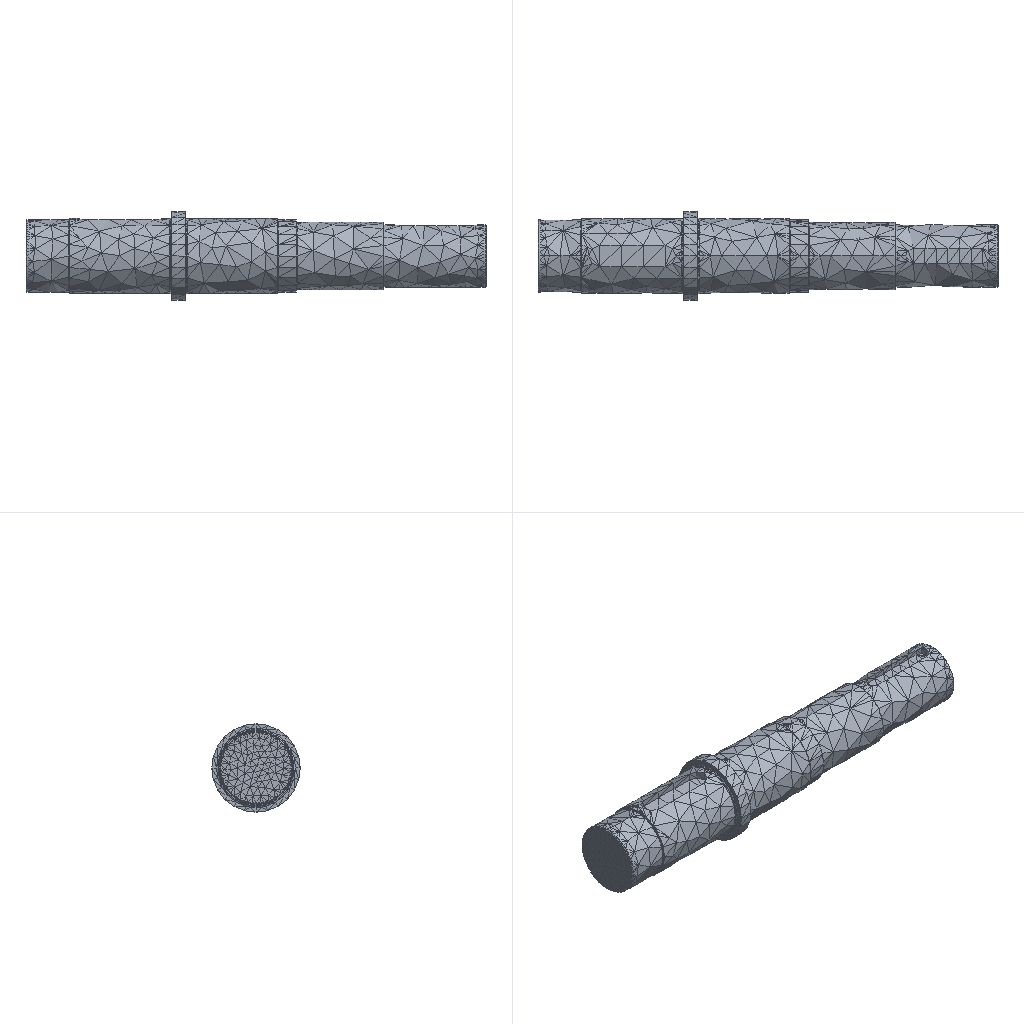Simulation study | ansys workbench
Ansys APDL input file, long lists of numbers shortened:
/batch
/config,noeldb,1     ! force off writing results to database
*get,_wallstrt,active,,time,wall
! ANSYS input file written by Workbench version 2022 R1
! File used for geometry attach: F:\ansys（分析文件汇总)\轴有限元分析222\优化后.STEP
/title,1--____ (C5)
! ****** Begin Custom Load Command Snippet ******
/COM, ACT Extensions:
/COM,     LSDYNA, 2021.1
/COM,
! ****** End   Custom Load Command Snippet ******
*DIM,_wb_ProjectScratch_dir,string,248
_wb_ProjectScratch_dir(1) = 'F:\ansys（分析文件汇总)\轴有限元分析222\_ProjectScratch\Scr8197\'
*DIM,_wb_SolverFiles_dir,string,248
_wb_SolverFiles_dir(1) = 'F:\ansys（分析文件汇总)\轴有限元分析222\1_files\dp0\SYS-1\MECH\'
*DIM,_wb_userfiles_dir,string,248
_wb_userfiles_dir(1) = 'F:\ansys（分析文件汇总)\轴有限元分析222\1_files\user_files\'
/com,--- Data in consistent NMM units. See Solving Units in the help system for more information.
/units,MPA
/nopr
/wb,file,start              !  signify a WB generated input file
/prep7
! Turn off shape checking because checks already performed inside WB mesher.
! See help system for more information.
SHPP,OFF,,NOWARN
/nolist
etcon,set             ! allow ANSYS to choose best KEYOP's for 180x elements, resets any applicable keyopt to MAPDL defaults
/com,*********** Nodes for the whole assembly ***********
nblock,3,,14791
(1i9,3e20.9e3)
        1     4.709807621E+01    -3.900000000E+01    -1.276756478E-12
! (13446 more lines like these left out)
-1
/com,*********** Nodes for all Remote Points ***********
nblock,3
(1i9,3e20.9e3)
    13448     2.171568898E+02     8.881784197E-16    -1.105137585E-15
-1
/wb,elem,start            !  set before creation of elements
/com,*********** Elements for Body 1 "___-FreeParts|____2[1]" ***********
et,1,187
eblock,19,solid,,7656
(19i9)
        1        1        1        1        0        0        0        0       10        0        1     1619     1746     2118     1971    11680    12397    11689    11688
! (15311 more lines like these left out)
-1
/wb,elem,end               !  done creating elements
/com,*********** Send User Defined Coordinate System(s) ***********
csys,0
toffst,273.15,  ! Temperature offset from absolute zero
/com,*********** Set Reference Temperature ***********
tref,22.
/wb,mat,start              !  starting to send materials
/com,*********** Send Materials ***********
Temperature = 'TEMP' ! Temperature
MP,DENS,1,7.85e-09,	! tonne mm^-3
MP,ALPX,1,1.2e-05,	! C^-1
MP,C,1,434000000,	! mm^2 s^-2 C^-1
MP,KXX,1,60.5,	! tonne mm s^-3 C^-1
MP,RSVX,1,0.00017,	! ohm mm
MP,EX,1,200000,	! tonne s^-2 mm^-1
MP,NUXY,1,0.3,
MP,MURX,1,10000,
/wb,mat,end                !  done sending materials
!************************* Model Summary ********************
!___-FreeParts|____2[1],	结构钢,	matid,	1
!************************* End Model Summary ********************
! get the diagonal of the bounding box. Needed later for other things
*get,_xmin,node,,mnloc,x
*get,_ymin,node,,mnloc,y
*get,_zmin,node,,mnloc,z
*get,_xmax,node,,mxloc,x
*get,_ymax,node,,mxloc,y
*get,_zmax,node,,mxloc,z
_ASMDIAG=(_xmax-_xmin)*(_xmax-_xmin)+(_ymax-_ymin)*(_ymax-_ymin)+(_zmax-_zmin)*(_zmax-_zmin)
_ASMDIAG=SQRT(_ASMDIAG)
/wb,contact,start          !  starting to send contact
/wb,contact,end            !  done creating contacts
/golist
/wb,load,start             !  starting to send loads
/com,*********** Fixed Supports ***********
CMBLOCK,_FIXEDSU,NODE,      955
(8i10)
         1         2         3         4        57        60        61        62
! (119 more lines like these left out)
cmsel,s,_FIXEDSU
d,all,all
nsel,all
/com,*********** Create Remote Point "内部远程点" ***********
! -------- Remote Point Used by "力矩" --------
*set,tid,3
*set,cid,2
et,cid,174
et,tid,170
keyo,tid,2,1               ! Don't fix the pilot node
keyo,tid,4,111111
keyo,cid,12,5              ! Bonded Contact
keyo,cid,4,1               ! Deformable RBE3 style load
keyo,cid,2,2               ! MPC style contact
eblock,10,,,513
(15i9)
    10698        2        2        2        0      472      473     1364     1364     5388     5392     1364     5389
! (512 more lines like these left out)
-1
*set,_npilot,13448
_npilot32=_npilot
type,tid
mat ,cid
real,cid
tshape,pilo
en,11211,_npilot
tshape
/com,*********** Construct Moment Using Remote Attachment ***********
/gst,on,on
fini
*get,_numnode,node,0,count
*get,_numelem,elem,0,count
*get, _MAXELEMNUM, elem, 0, NUM, MAX
*get, _MAXNODENUM, node, 0, NUM, MAX
*get, _MAXELEMTYPE, etyp, 0, NUM, MAX
*get, _MAXREALCONST, real, 0, NUM, MAX
/go
/wb,load,end               !  done creating loads
/com,--- Number of total nodes = %_numnode%
/com,--- Number of contact elements = 513
/com,--- Number of spring elements = 0
/com,--- Number of bearing elements = 0
/com,--- Number of solid elements = 7656
/com,--- Number of condensed parts = 0
/com,--- Number of total elements = %_numelem%
*get,_wallbsol,active,,time,wall
/com,****************************************************************************
/com,*************************    SOLUTION       ********************************
/com,****************************************************************************
/solu
antype,0                   ! static analysis
_thickRatio=  1     ! Ratio of thick parts in the model
eqsl,pcg,1e-8,,,,,,1
cntr,print,1               ! print out contact info and also make no initial contact an error
dmpoption,emat,no             ! Don't combine emat file for DANSYS
dmpoption,esav,no             ! Don't combine esav file for DANSYS
nldiag,cont,iter           ! print out contact info each equilibrium iteration
rescontrol,,none                 ! Do not keep any restart files
/com,****************************************************
/com,******************* SOLVE FOR LS 1 OF 1 ****************
nsel,s,node,,13448
f,all,mx,900000.
f,all,my,0.
f,all,mz,0.
nsel,all
/nopr
/gopr
nsub,1,1,1
time,1.
outres,erase
outres,all,none
outres,nsol,all,
outres,rsol,all
outres,eangl,all
outres,etmp,all
outres,veng,all
outres,strs,all,
outres,epel,all,
outres,eppl,all,
outres,cont,all,
! *********** WB SOLVE COMMAND ***********
! check interactive state
*get,ANSINTER_,active,,int
*if,ANSINTER_,ne,0,then
/eof
*endif
solve
/com *************** Write FE CONNECTORS *********
CEWRITE,file,ce,,INTE
/com,****************************************************
/com,*************** FINISHED SOLVE FOR LS 1 *************
*get,_wallasol,active,,time,wall
/nopr
*get,_numnode,node,0,count
*get,_numelem,elem,0,count
*get, _MAXELEMNUM, elem, 0, NUM, MAX
*get, _MAXNODENUM, node, 0, NUM, MAX,,,INTERNAL
*get, _MAXELEMTYPE, etyp, 0, NUM, MAX
*get, _MAXREALCONST, real, 0, NUM, MAX
/gopr
*get,_PCGITER,active,,solu,cgiter
/post1
xmlo,ENCODING,ISO-8859-1
xmlo,parm
/xml,parm,xml
fini
/gopr
*get,_walldone,active,,time,wall
_preptime=(_wallbsol-_wallstrt)*3600
_solvtime=(_wallasol-_wallbsol)*3600
_posttime=(_walldone-_wallasol)*3600
_totaltim=(_walldone-_wallstrt)*3600
*get,_dlbratio,active,0,solu,dlbr
*get,_combtime,active,0,solu,comb
*get,_ssmode,active,0,solu,ssmm
*get,_ndofs,active,0,solu,ndof
*get,_sol_end_time,active,0,set,time
*if,_sol_end_time,eq,1.,then
/fclean				!clean distributed files
*endif
/com,--- Total number of nodes = %_numnode%
/com,--- Total number of elements = %_numelem%
/com,--- Element load balance ratio = %_dlbratio%
/com,--- Time to combine distributed files = %_combtime%
/com,--- Sparse memory mode = %_ssmode%
/com,--- Number of DOF = %_ndofs%
/wb,file,end               ! done with WB generated input